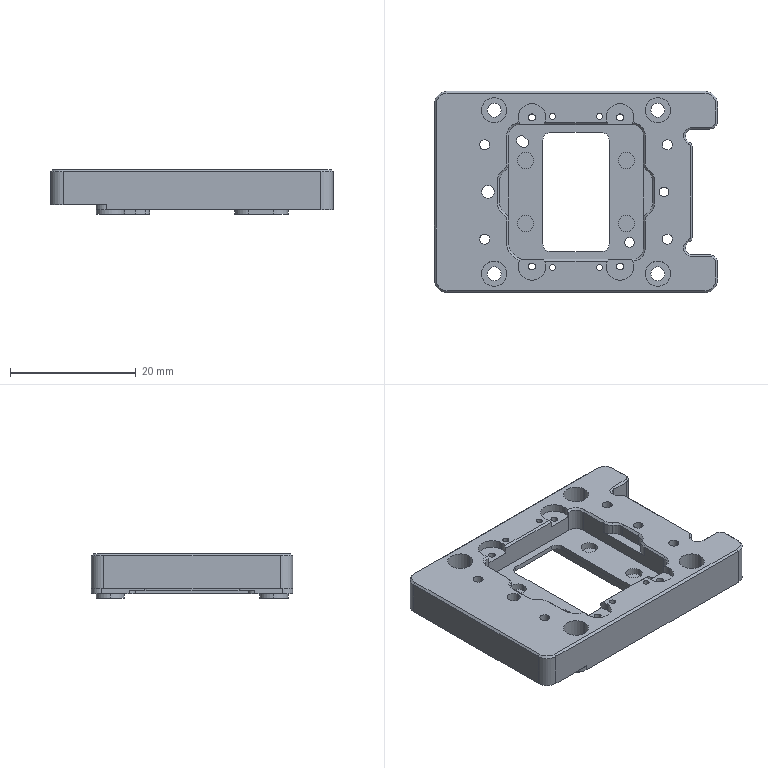NC program | NX | posted with a generic post | part box 45 x 32 x 7.05 mm
Lines 1 to 1919 of 2540, first 1706 of 1901 lines:
N10 G17 G21 G94 G90
(FLOOR_WALL_COPY , TOOL : D63)
N12 T03 M6
N14 G54
N16 G17 G0 G90 X-57. Y0. S6500 M3
N18 G43 Z30. H3
N20 Z5.
N22 G94 G1 Z2. F1250.
N24 X-54.
N26 X54.
N28 X57.
N30 Z5.
N32 G0 Z30.
N34 X-57.
N36 Z4.
N38 G1 Z1.
N40 X-54.
N42 X54.
N44 X57.
N46 Z4.
N48 G0 Z30.
N50 X-57.
N52 Z3.
N54 G1 Z0.
N56 X-54.
N58 X54.
N60 X57.
N62 Z3.
N64 G0 Z30.
N66 M5
(DRILLING_COPY_1 , TOOL : D6A45)
N68 T01 M6
N70 G54
N72 G17 G0 G90 X8.987 Y12.964 S5000 M3
N74 G43 Z30. H1
N76 G94 G81 G98 Z-0.6 F250. R3.
N78 X-9.013 Y-13.028
N80 G80
N82 G0 X-9.013 Y-13.028 Z30.
N84 M5
(DRILLING_COPY_COPY_1_COPY_COPY_1 , TOOL : 1.17ZT)
N86 T18 M6
N88 G54
N90 G17 G0 G90 X8.987 Y12.964 S2000 M3
N92 G43 Z30. H18
N94 G94 G83 G98 Z-3.352 F100. Q1. R3.
N96 X-9.013 Y-13.028
N98 G80
N100 G0 X-9.013 Y-13.028 Z30.
N102 M5
(FLOOR_WALL_2 , TOOL : D6)
N104 T06 M6
N106 G54
N108 G17 G0 G90 X1.501 Y-21.097 S9500 M3
N110 G43 Z30. H6
N112 Z0.7
N114 G94 G1 Z-0.3 F1000.
N116 X0.52 Y-19.397
N118 G3 X0. Y-19.097 R0.6
N120 G1 X-20.5 F2500.
N122 G2 X-25.597 Y-14. R5.097
N124 G1 Y-11.214
N126 G2 X-24.397 Y-8.317 R4.097
N128 G1 X-24.183 Y-8.103
N130 G2 X-21.597 Y-6.915 R4.097
N132 G1 Y6.915
N134 G2 X-24.183 Y8.103 R4.097
N136 G1 X-24.397 Y8.317
N138 G2 X-25.597 Y11.214 R4.097
N140 G1 Y14.
N142 G2 X-20.5 Y19.097 R5.097
N144 G1 X20.5
N146 G2 X25.597 Y14. R5.097
N148 G1 Y-14.
N150 G2 X20.5 Y-19.097 R5.097
N152 G1 X0.
N154 Y-16.097
N156 X-3.94
N158 G3 X-3.309 Y-11.355 R5.95
N160 X-3.948 Y-10.105 R3.7
N162 X-4.701 Y-8.92 R3.7
N164 X-9.025 Y-7.058 R5.95
N166 G1 X-13.025
N168 G3 X-18.11 Y-16.097 R5.95
N170 G1 X-17.597 Y-15.786
N172 G2 X-13.025 Y-7.658 R5.35
N174 G1 X-9.025
N176 G2 X-5.137 Y-9.332 R5.35
N178 X-4.475 Y-10.406 R3.1
N180 X-3.886 Y-11.521 R3.1
N182 X-9.025 Y-18.358 R5.35
N184 G1 X-13.025
N186 G2 X-17.597 Y-15.786 R5.35
N188 G1 X-18.11 Y-16.097
N190 X-20.5
N192 G2 X-22.597 Y-14. R2.097
N194 G1 Y-11.214
N196 G2 X-22.276 Y-10.439 R1.097
N198 G1 X-22.061 Y-10.224
N200 G2 X-21.369 Y-9.906 R1.097
N202 G3 X-18.597 Y-6.915 R3.
N204 G1 Y6.915
N206 G3 X-21.369 Y9.906 R3.
N208 G2 X-22.061 Y10.224 R1.097
N210 G1 X-22.276 Y10.439
N212 G2 X-22.597 Y11.214 R1.097
N214 G1 Y14.
N216 G2 X-20.5 Y16.097 R2.097
N218 G1 X-18.098
N220 G3 X-7.953 Y16.097 R-5.95
N222 G1 X-8.464 Y15.783
N224 G2 X-10.23 Y8.426 R5.35
N226 X-8.464 Y15.783 R-5.35
N228 G1 X-7.953 Y16.097
N230 X3.912
N232 G3 X3.257 Y11.359 R5.95
N234 X3.907 Y10.083 R3.7
N236 X4.677 Y8.874 R3.7
N238 X8.981 Y7.032 R5.95
N240 G1 X12.981
N242 G3 X18.051 Y16.097 R5.95
N244 G1 X17.54 Y15.783
N246 G2 X12.981 Y7.632 R5.35
N248 G1 X8.981
N250 G2 X5.111 Y9.288 R5.35
N252 X4.435 Y10.384 R3.1
N254 X3.834 Y11.523 R3.1
N256 X8.981 Y18.332 R5.35
N258 G1 X12.981
N260 G2 X17.54 Y15.783 R5.35
N262 G1 X18.051 Y16.097
N264 X20.5
N266 G2 X22.597 Y14. R2.097
N268 G1 Y-14.
N270 G2 X20.5 Y-16.097 R2.097
N272 G1 X18.063
N274 G3 X7.888 Y-16.097 R-5.95
N276 G1 X8.401 Y-15.786
N278 G2 X10.201 Y-8.437 R5.35
N280 X8.401 Y-15.786 R-5.35
N282 G1 X7.888 Y-16.097
N284 X0.
N286 Y-13.097
N288 X-0.075
N290 G3 X-0.427 Y-10.521 R8.95
N292 X-1.329 Y-8.607 R6.7
N294 X-2.522 Y-6.859 R6.7
N296 X-9.025 Y-4.058 R8.95
N298 G1 X-13.025
N300 G3 X-15.597 Y-4.436 R8.95
N302 G1 Y4.415
N304 G3 X-4.076 Y12.987 R8.95
N306 G1 Y13.097
N308 X0.032
N310 G3 X0.371 Y10.541 R8.95
N312 X1.287 Y8.585 R6.7
N314 X2.507 Y6.803 R6.7
N316 X8.981 Y4.032 R8.95
N318 G1 X12.981
N320 G3 X19.597 Y6.954 R8.95
N322 G1 Y-6.989
N324 G3 X4.026 Y-13.011 R8.95
N326 G1 Y-13.097
N328 X0.
N330 X1.965 Y-8.365
N332 G3 X1.281 Y-7.114 R9.7
N334 X-0.342 Y-4.798 R9.7
N336 X-9.025 Y-1.058 R11.95
N338 G1 X-12.597
N340 Y1.045
N342 G3 X-2.012 Y8.35 R11.95
N344 X-1.323 Y7.093 R9.7
N346 X0.337 Y4.731 R9.7
N348 X8.981 Y1.032 R11.95
N350 G1 X12.981
N352 G3 X16.597 Y1.592 R11.95
N354 G1 Y-1.623
N356 G3 X1.965 Y-8.365 R11.95
N358 G1 X1.976 Y-2.886
N360 G3 X-3.997 Y1.071 R14.95
N362 X-2.024 Y2.865 R14.95
N364 X-1.833 Y2.66 R12.7
N366 X3.947 Y-1.095 R14.95
N368 X1.976 Y-2.886 R14.95
N370 X1.845 Y-3.471 R0.6
N372 G1 Z0.7
N374 G0 X1.501 Y-21.097 Z0.4
N376 G1 Z-0.6 F1000.
N378 X0.52 Y-19.397
N380 G3 X0. Y-19.097 R0.6
N382 G1 X-20.5 F2500.
N384 G2 X-25.597 Y-14. R5.097
N386 G1 Y-11.214
N388 G2 X-24.397 Y-8.317 R4.097
N390 G1 X-24.183 Y-8.103
N392 G2 X-21.597 Y-6.915 R4.097
N394 G1 Y6.915
N396 G2 X-24.183 Y8.103 R4.097
N398 G1 X-24.397 Y8.317
N400 G2 X-25.597 Y11.214 R4.097
N402 G1 Y14.
N404 G2 X-20.5 Y19.097 R5.097
N406 G1 X20.5
N408 G2 X25.597 Y14. R5.097
N410 G1 Y-14.
N412 G2 X20.5 Y-19.097 R5.097
N414 G1 X0.
N416 Y-16.097
N418 X-3.94
N420 G3 X-3.309 Y-11.355 R5.95
N422 X-3.948 Y-10.105 R3.7
N424 X-4.701 Y-8.92 R3.7
N426 X-9.025 Y-7.058 R5.95
N428 G1 X-13.025
N430 G3 X-18.11 Y-16.097 R5.95
N432 G1 X-17.597 Y-15.786
N434 G2 X-13.025 Y-7.658 R5.35
N436 G1 X-9.025
N438 G2 X-5.137 Y-9.332 R5.35
N440 X-4.475 Y-10.406 R3.1
N442 X-3.886 Y-11.521 R3.1
N444 X-9.025 Y-18.358 R5.35
N446 G1 X-13.025
N448 G2 X-17.597 Y-15.786 R5.35
N450 G1 X-18.11 Y-16.097
N452 X-20.5
N454 G2 X-22.597 Y-14. R2.097
N456 G1 Y-11.214
N458 G2 X-22.276 Y-10.439 R1.097
N460 G1 X-22.061 Y-10.224
N462 G2 X-21.369 Y-9.906 R1.097
N464 G3 X-18.597 Y-6.915 R3.
N466 G1 Y6.915
N468 G3 X-21.369 Y9.906 R3.
N470 G2 X-22.061 Y10.224 R1.097
N472 G1 X-22.276 Y10.439
N474 G2 X-22.597 Y11.214 R1.097
N476 G1 Y14.
N478 G2 X-20.5 Y16.097 R2.097
N480 G1 X-18.098
N482 G3 X-7.953 Y16.097 R-5.95
N484 G1 X-8.464 Y15.783
N486 G2 X-10.23 Y8.426 R5.35
N488 X-8.464 Y15.783 R-5.35
N490 G1 X-7.953 Y16.097
N492 X3.912
N494 G3 X3.257 Y11.359 R5.95
N496 X3.907 Y10.083 R3.7
N498 X4.677 Y8.874 R3.7
N500 X8.981 Y7.032 R5.95
N502 G1 X12.981
N504 G3 X18.051 Y16.097 R5.95
N506 G1 X17.54 Y15.783
N508 G2 X12.981 Y7.632 R5.35
N510 G1 X8.981
N512 G2 X5.111 Y9.288 R5.35
N514 X4.435 Y10.384 R3.1
N516 X3.834 Y11.523 R3.1
N518 X8.981 Y18.332 R5.35
N520 G1 X12.981
N522 G2 X17.54 Y15.783 R5.35
N524 G1 X18.051 Y16.097
N526 X20.5
N528 G2 X22.597 Y14. R2.097
N530 G1 Y-14.
N532 G2 X20.5 Y-16.097 R2.097
N534 G1 X18.063
N536 G3 X7.888 Y-16.097 R-5.95
N538 G1 X8.401 Y-15.786
N540 G2 X10.201 Y-8.437 R5.35
N542 X8.401 Y-15.786 R-5.35
N544 G1 X7.888 Y-16.097
N546 X0.
N548 Y-13.097
N550 X-0.075
N552 G3 X-0.427 Y-10.521 R8.95
N554 X-1.329 Y-8.607 R6.7
N556 X-2.522 Y-6.859 R6.7
N558 X-9.025 Y-4.058 R8.95
N560 G1 X-13.025
N562 G3 X-15.597 Y-4.436 R8.95
N564 G1 Y4.415
N566 G3 X-4.076 Y12.987 R8.95
N568 G1 Y13.097
N570 X0.032
N572 G3 X0.371 Y10.541 R8.95
N574 X1.287 Y8.585 R6.7
N576 X2.507 Y6.803 R6.7
N578 X8.981 Y4.032 R8.95
N580 G1 X12.981
N582 G3 X19.597 Y6.954 R8.95
N584 G1 Y-6.989
N586 G3 X4.026 Y-13.011 R8.95
N588 G1 Y-13.097
N590 X0.
N592 X1.965 Y-8.365
N594 G3 X1.281 Y-7.114 R9.7
N596 X-0.342 Y-4.798 R9.7
N598 X-9.025 Y-1.058 R11.95
N600 G1 X-12.597
N602 Y1.045
N604 G3 X-2.012 Y8.35 R11.95
N606 X-1.323 Y7.093 R9.7
N608 X0.337 Y4.731 R9.7
N610 X8.981 Y1.032 R11.95
N612 G1 X12.981
N614 G3 X16.597 Y1.592 R11.95
N616 G1 Y-1.623
N618 G3 X1.965 Y-8.365 R11.95
N620 G1 X1.976 Y-2.886
N622 G3 X-3.997 Y1.071 R14.95
N624 X-2.024 Y2.865 R14.95
N626 X-1.833 Y2.66 R12.7
N628 X3.947 Y-1.095 R14.95
N630 X1.976 Y-2.886 R14.95
N632 X1.845 Y-3.471 R0.6
N634 G1 Z0.4
N636 G0 X27.597 Y1.501 Z0.15
N638 G1 Z-0.85 F1000.
N640 X25.897 Y0.52
N642 G3 X25.597 Y0. R0.6
N644 G1 Y-14. F2500.
N646 G2 X20.5 Y-19.097 R5.097
N648 G1 X14.187
N650 Y-19.067
N652 G3 X18.331 Y-14.4 R4.7
N654 G1 Y-10.
N656 G3 X14.231 Y-5.9 R4.1
N658 G1 X6.95
N660 G3 X2.85 Y-10. R4.1
N662 G1 Y-11.112
N664 G3 X0.281 Y-12.284 R4.1
N666 G2 X-0.281 Y-12.284 R0.4
N668 G3 X-2.85 Y-11.112 R4.1
N670 G1 Y11.112
N672 G3 X-0.281 Y12.284 R4.1
N674 G2 X0.281 Y12.284 R0.4
N676 G3 X2.85 Y11.112 R4.1
N678 G1 Y10.
N680 G3 X6.95 Y5.9 R4.1
N682 G1 X14.231
N684 G3 X18.331 Y10. R4.1
N686 G1 Y14.4
N688 G3 X14.187 Y19.067 R4.7
N690 G1 Y19.097
N692 X20.5
N694 G2 X25.597 Y14. R5.097
N696 G1 Y0.
N698 X22.597
N700 Y-14.
N702 G2 X21.166 Y-15.989 R2.097
N704 G3 X21.331 Y-14.4 R7.7
N706 G1 Y-10.
N708 G3 X14.231 Y-2.9 R7.1
N710 G1 X6.95
N712 G3 X0.15 Y-7.958 R7.1
N714 G1 Y7.958
N716 G3 X5.953 Y2.97 R7.1
N718 G1 X5.532 Y0.
N720 G3 X3.15 Y-0.642 R10.1
N722 G1 Y0.642
N724 G3 X5.532 Y0. R10.1
N726 G1 X5.953 Y2.97
N728 G3 X6.95 Y2.9 R7.1
N730 G1 X14.231
N732 G3 X21.331 Y10. R7.1
N734 G1 Y14.4
N736 G3 X21.166 Y15.989 R7.7
N738 G2 X22.597 Y14. R2.097
N740 G1 Y0.
N742 X19.597
N744 Y-1.443
N746 G3 X15.649 Y0. R10.1
N748 X19.597 Y1.443 R10.1
N750 G1 Y0.
N752 G3 X19.897 Y-0.52 R0.6
N754 G1 Z0.15
N756 G0 X27.597 Y1.501 Z-0.1
N758 G1 Z-1.1 F1000.
N760 X25.897 Y0.52
N762 G3 X25.597 Y0. R0.6
N764 G1 Y-14. F2500.
N766 G2 X20.5 Y-19.097 R5.097
N768 G1 X14.187
N770 Y-19.067
N772 G3 X18.331 Y-14.4 R4.7
N774 G1 Y-10.
N776 G3 X14.231 Y-5.9 R4.1
N778 G1 X6.95
N780 G3 X2.887 Y-9.453 R4.1
N782 X-2.85 Y-9.412 R3.85
N784 G1 Y9.412
N786 G3 X2.887 Y9.453 R3.85
N788 X6.95 Y5.9 R4.1
N790 G1 X14.231
N792 G3 X18.331 Y10. R4.1
N794 G1 Y14.4
N796 G3 X14.187 Y19.067 R4.7
N798 G1 Y19.097
N800 X20.5
N802 G2 X25.597 Y14. R5.097
N804 G1 Y0.
N806 X22.597
N808 Y-14.
N810 G2 X21.166 Y-15.989 R2.097
N812 G3 X21.331 Y-14.4 R7.7
N814 G1 Y-10.
N816 G3 X14.231 Y-2.9 R7.1
N818 G1 X6.95
N820 G3 X1.595 Y-5.338 R7.1
N822 X0.15 Y-5.152 R6.85
N824 G1 Y5.152
N826 G3 X1.595 Y5.338 R6.85
N828 X5.953 Y2.97 R7.1
N830 G1 X5.532 Y0.
N832 G3 X3.15 Y-0.642 R10.1
N834 G1 Y0.642
N836 G3 X5.532 Y0. R10.1
N838 G1 X5.953 Y2.97
N840 G3 X6.95 Y2.9 R7.1
N842 G1 X14.231
N844 G3 X21.331 Y10. R7.1
N846 G1 Y14.4
N848 G3 X21.166 Y15.989 R7.7
N850 G2 X22.597 Y14. R2.097
N852 G1 Y0.
N854 X19.597
N856 Y-1.443
N858 G3 X15.649 Y0. R10.1
N860 X19.597 Y1.443 R10.1
N862 G1 Y0.
N864 G3 X19.897 Y-0.52 R0.6
N866 G1 Z-0.1
N868 G0 X27.597 Y1.501 Z-0.4
N870 G1 Z-1.4 F1000.
N872 X25.897 Y0.52
N874 G3 X25.597 Y0. R0.6
N876 G1 Y-14. F2500.
N878 G2 X20.5 Y-19.097 R5.097
N880 G1 X14.187
N882 Y-19.067
N884 G3 X18.331 Y-14.4 R4.7
N886 G1 Y-7.824
N888 G3 X18.314 Y-7.5 R3.1
N890 X18.331 Y-7.176 R3.1
N892 G1 Y7.176
N894 G3 X18.314 Y7.5 R3.1
N896 X18.331 Y7.824 R3.1
N898 G1 Y14.4
N900 G3 X14.187 Y19.067 R4.7
N902 G1 Y19.097
N904 X20.5
N906 G2 X25.597 Y14. R5.097
N908 G1 Y0.
N910 X22.597
N912 Y-14.
N914 G2 X21.166 Y-15.989 R2.097
N916 G3 X21.331 Y-14.4 R7.7
N918 G1 Y-7.824
N920 G3 X21.323 Y-7.5 R6.1
N922 X21.331 Y-7.176 R6.1
N924 G1 Y7.176
N926 G3 X21.323 Y7.5 R6.1
N928 X21.331 Y7.824 R6.1
N930 G1 Y14.4
N932 G3 X21.166 Y15.989 R7.7
N934 G2 X22.597 Y14. R2.097
N936 G1 Y0.
N938 G3 X22.897 Y-0.52 R0.6
N940 G1 X27.597
N942 Z-0.4
N944 G0 Z30.
N946 X2.55
N948 Z-0.4
N950 G1 Z-1.4 F1000.
N952 G3 X2.85 Y0. R0.6
N954 G1 Y-9.412 F2500.
N956 G3 X-2.85 Y-9.412 R3.85
N958 G1 Y9.412
N960 G3 X2.85 Y9.412 R3.85
N962 G1 Y0.
N964 X0.15
N966 Y-5.452
N968 G3 X-0.15 Y-5.452 R6.55
N970 G1 Y5.452
N972 G3 X0.15 Y5.452 R6.55
N974 G1 Y0.
N976 G3 X0.45 Y-0.52 R0.6
N978 G1 Z-0.4
N980 G0 Z30.
N982 X-23.597 Y-1.501
N984 Z0.15
N986 G1 Z-0.85 F1000.
N988 X-21.897 Y-0.52
N990 G3 X-21.597 Y0. R0.6
N992 G1 Y6.912 F2500.
N994 G3 X-21.286 Y6.9 R4.1
N996 G1 X-19.394
N998 G3 X-16.711 Y5.9 R4.1
N1000 G1 X-12.464
N1002 Y-5.9
N1004 X-16.711
N1006 G3 X-19.394 Y-6.9 R4.1
N1008 G1 X-21.286
N1010 G3 X-21.597 Y-6.912 R4.1
N1012 G1 Y0.
N1014 X-18.597
N1016 Y3.155
N1018 G3 X-16.711 Y2.9 R7.1
N1020 G1 X-15.464
N1022 Y-2.9
N1024 X-16.711
N1026 G3 X-18.597 Y-3.155 R7.1
N1028 G1 Y0.
N1030 G3 X-18.897 Y0.52 R0.6
N1032 G1 X-23.597
N1034 Z0.15
N1036 G0 Y-1.501 Z-0.1
N1038 G1 Z-1.1 F1000.
N1040 X-21.897 Y-0.52
N1042 G3 X-21.597 Y0. R0.6
N1044 G1 Y6.912 F2500.
N1046 G3 X-21.286 Y6.9 R4.1
N1048 G1 X-19.394
N1050 G3 X-16.711 Y5.9 R4.1
N1052 G1 X-12.464
N1054 Y-5.9
N1056 X-16.711
N1058 G3 X-19.394 Y-6.9 R4.1
N1060 G1 X-21.286
N1062 G3 X-21.597 Y-6.912 R4.1
N1064 G1 Y0.
N1066 X-18.597
N1068 Y3.155
N1070 G3 X-16.711 Y2.9 R7.1
N1072 G1 X-15.464
N1074 Y-2.9
N1076 X-16.711
N1078 G3 X-18.597 Y-3.155 R7.1
N1080 G1 Y0.
N1082 G3 X-18.897 Y0.52 R0.6
N1084 G1 X-23.597
N1086 Z-0.1
N1088 G0 Z30.
N1090 X-2.55
N1092 Z-1.05
N1094 G1 Z-2.05 F1000.
N1096 G3 X-2.85 Y0. R0.6
N1098 G1 Y9.412 F2500.
N1100 G3 X2.85 Y9.412 R3.85
N1102 G1 Y-9.412
N1104 G3 X-2.85 Y-9.412 R3.85
N1106 G1 Y0.
N1108 X-0.15
N1110 Y5.452
N1112 G3 X0.15 Y5.452 R6.55
N1114 G1 Y-5.452
N1116 G3 X-0.15 Y-5.452 R6.55
N1118 G1 Y0.
N1120 G3 X-0.45 Y0.52 R0.6
N1122 G1 Z-1.05
N1124 G0 X-2.55 Z-1.35
N1126 G1 Z-2.35 F1000.
N1128 G3 X-2.85 Y0. R0.6
N1130 G1 Y9.412 F2500.
N1132 G3 X2.85 Y9.412 R3.85
N1134 G1 Y-9.412
N1136 G3 X-2.85 Y-9.412 R3.85
N1138 G1 Y0.
N1140 X-0.15
N1142 Y5.452
N1144 G3 X0.15 Y5.452 R6.55
N1146 G1 Y-5.452
N1148 G3 X-0.15 Y-5.452 R6.55
N1150 G1 Y0.
N1152 G3 X-0.45 Y0.52 R0.6
N1154 G1 Z-1.35
N1156 G0 Z30.
N1158 M5
(CAVITY_MILL_COPY_1 , TOOL : D3)
N1160 T17 M6
N1162 G54
N1164 G17 G0 G90 X-13.36 Y-6.9 S9500 M3
N1166 G43 Z30. H17
N1168 Z-0.95
N1170 G94 G1 X-13.302 Y-7. F1100.
N1172 G3 X-12.436 Y-7.5 R1.
N1174 G1 X-10.864
N1176 Y-5.928
N1178 G3 X-11.364 Y-5.062 R1.
N1180 G1 X-11.464 Y-5.005
N1182 G0 X-13.36 Y-6.9 Z-1.2
N1184 G1 X-13.302 Y-7.
N1186 G3 X-12.436 Y-7.5 R1.
N1188 G1 X-10.864
N1190 Y-5.928
N1192 G3 X-11.364 Y-5.062 R1.
N1194 G1 X-11.464 Y-5.005
N1196 G0 Z30.
N1198 Y5.005
N1200 Z-0.95
N1202 G1 X-11.364 Y5.062
N1204 G3 X-10.864 Y5.928 R1.
N1206 G1 Y7.5
N1208 X-12.436
N1210 G3 X-13.302 Y7. R1.
N1212 G1 X-13.36 Y6.9
N1214 G0 X-11.464 Y5.005 Z-1.2
N1216 G1 X-11.364 Y5.062
N1218 G3 X-10.864 Y5.928 R1.
N1220 G1 Y7.5
N1222 X-12.436
N1224 G3 X-13.302 Y7. R1.
N1226 G1 X-13.36 Y6.9
N1228 G0 Z30.
(CAVITY_MILL_COPY_1_COPY , TOOL : D3)
N1230 X-1.435 Y9.605
N1232 Z-0.992
N1234 G3 X-1.644 Y10.55 R1.
N1236 G2 X-1.94 Y13.02 R2.192
N1238 X-3.164 Y12.7 R2.5
N1240 G1 X-4.25
N1242 G3 X-4.45 Y12.5 R0.2
N1244 G1 Y9.709
N1246 G3 X-3.95 Y8.843 R1.
N1248 G1 X-3.85 Y8.785
N1250 G0 X-1.436 Y9.538 Z-1.283
N1252 G3 X-1.661 Y10.482 R1.
N1254 G2 X-2.029 Y12.972 R2.25
N1256 X-3.164 Y12.7 R2.5
N1258 G1 X-4.25
N1260 G3 X-4.45 Y12.5 R0.2
N1262 G1 Y9.613
N1264 G3 X-3.95 Y8.747 R1.
N1266 G1 X-3.85 Y8.69
N1268 G0 X-1.436 Y9.538 Z-1.575
N1270 G3 X-1.661 Y10.482 R1.
N1272 G2 X-2.029 Y12.972 R2.25
N1274 X-3.164 Y12.7 R2.5
N1276 G1 X-4.25
N1278 G3 X-4.45 Y12.5 R0.2
N1280 G1 Y9.613
N1282 G3 X-3.95 Y8.747 R1.
N1284 G1 X-3.85 Y8.69
N1286 G0 X-1.436 Y9.538 Z-1.867
N1288 G3 X-1.661 Y10.482 R1.
N1290 G2 X-2.029 Y12.972 R2.25
N1292 X-3.164 Y12.7 R2.5
N1294 G1 X-4.25
N1296 G3 X-4.45 Y12.5 R0.2
N1298 G1 Y9.613
N1300 G3 X-3.95 Y8.747 R1.
N1302 G1 X-3.85 Y8.69
N1304 G0 X-1.436 Y9.538 Z-2.158
N1306 G3 X-1.661 Y10.482 R1.
N1308 G2 X-2.029 Y12.972 R2.25
N1310 X-3.164 Y12.7 R2.5
N1312 G1 X-4.25
N1314 G3 X-4.45 Y12.5 R0.2
N1316 G1 Y9.613
N1318 G3 X-3.95 Y8.747 R1.
N1320 G1 X-3.85 Y8.69
N1322 G0 X-1.436 Y9.538 Z-2.45
N1324 G3 X-1.661 Y10.482 R1.
N1326 G2 X-2.029 Y12.972 R2.25
N1328 X-3.164 Y12.7 R2.5
N1330 G1 X-4.25
N1332 G3 X-4.45 Y12.5 R0.2
N1334 G1 Y9.613
N1336 G3 X-3.95 Y8.747 R1.
N1338 G1 X-3.85 Y8.69
N1340 G0 Z30.
N1342 X4.077 Y8.836
N1344 Z-0.992
N1346 G3 X4.464 Y9.736 R1.
N1348 G2 X4.45 Y10. R2.5
N1350 G1 Y12.5
N1352 G3 X4.25 Y12.7 R0.2
N1354 G1 X3.164
N1356 G2 X1.94 Y13.02 R2.5
N1358 X1.647 Y10.554 R2.192
N1360 G3 X1.441 Y9.609 R1.
N1362 G0 X3.85 Y8.69 Z-1.283
N1364 G1 X3.95 Y8.747
N1366 G3 X4.45 Y9.613 R1.
N1368 G1 Y12.5
N1370 G3 X4.25 Y12.7 R0.2
N1372 G1 X3.164
N1374 G2 X2.029 Y12.972 R2.5
N1376 X1.661 Y10.482 R2.25
N1378 G3 X1.436 Y9.538 R1.
N1380 G0 X3.85 Y8.69 Z-1.575
N1382 G1 X3.95 Y8.747
N1384 G3 X4.45 Y9.613 R1.
N1386 G1 Y12.5
N1388 G3 X4.25 Y12.7 R0.2
N1390 G1 X3.164
N1392 G2 X2.029 Y12.972 R2.5
N1394 X1.661 Y10.482 R2.25
N1396 G3 X1.436 Y9.538 R1.
N1398 G0 X3.85 Y8.69 Z-1.867
N1400 G1 X3.95 Y8.747
N1402 G3 X4.45 Y9.613 R1.
N1404 G1 Y12.5
N1406 G3 X4.25 Y12.7 R0.2
N1408 G1 X3.164
N1410 G2 X2.029 Y12.972 R2.5
N1412 X1.661 Y10.482 R2.25
N1414 G3 X1.436 Y9.538 R1.
N1416 G0 X3.85 Y8.69 Z-2.158
N1418 G1 X3.95 Y8.747
N1420 G3 X4.45 Y9.613 R1.
N1422 G1 Y12.5
N1424 G3 X4.25 Y12.7 R0.2
N1426 G1 X3.164
N1428 G2 X2.029 Y12.972 R2.5
N1430 X1.661 Y10.482 R2.25
N1432 G3 X1.436 Y9.538 R1.
N1434 G0 X3.85 Y8.69 Z-2.45
N1436 G1 X3.95 Y8.747
N1438 G3 X4.45 Y9.613 R1.
N1440 G1 Y12.5
N1442 G3 X4.25 Y12.7 R0.2
N1444 G1 X3.164
N1446 G2 X2.029 Y12.972 R2.5
N1448 X1.661 Y10.482 R2.25
N1450 G3 X1.436 Y9.538 R1.
N1452 G0 Z30.
N1454 X1.441 Y-9.609
N1456 Z-0.992
N1458 G3 X1.647 Y-10.554 R1.
N1460 G2 X1.94 Y-13.02 R2.192
N1462 X3.164 Y-12.7 R2.5
N1464 G1 X3.629
N1466 X3.717 Y-12.712
N1468 X3.77 Y-12.641
N1470 X4.391 Y-12.02
N1472 X4.462 Y-11.967
N1474 X4.45 Y-11.879
N1476 Y-10.
N1478 G2 X4.464 Y-9.736 R2.5
N1480 G3 X4.077 Y-8.836 R1.
N1482 G0 X1.436 Y-9.538 Z-1.283
N1484 G3 X1.661 Y-10.482 R1.
N1486 G2 X2.056 Y-12.915 R2.25
N1488 G1 X2.04 Y-12.967
N1490 G2 X3.164 Y-12.7 R2.5
N1492 G1 X3.629
N1494 X3.717 Y-12.712
N1496 X3.77 Y-12.641
N1498 X4.391 Y-12.02
N1500 X4.462 Y-11.967
N1502 X4.45 Y-11.879
N1504 Y-9.613
N1506 G3 X3.95 Y-8.747 R1.
N1508 G1 X3.85 Y-8.69
N1510 G0 X1.436 Y-9.538 Z-1.575
N1512 G3 X1.661 Y-10.482 R1.
N1514 G2 X2.056 Y-12.915 R2.25
N1516 G1 X2.041 Y-12.966
N1518 G2 X3.164 Y-12.7 R2.5
N1520 G1 X3.629
N1522 X3.717 Y-12.712
N1524 X3.77 Y-12.641
N1526 X4.391 Y-12.02
N1528 X4.462 Y-11.967
N1530 X4.45 Y-11.879
N1532 Y-9.613
N1534 G3 X3.95 Y-8.747 R1.
N1536 G1 X3.85 Y-8.69
N1538 G0 X1.436 Y-9.538 Z-1.867
N1540 G3 X1.661 Y-10.482 R1.
N1542 G2 X2.056 Y-12.915 R2.25
N1544 G1 X2.042 Y-12.966
N1546 G2 X3.164 Y-12.7 R2.5
N1548 G1 X3.629
N1550 X3.717 Y-12.712
N1552 X3.77 Y-12.641
N1554 X4.391 Y-12.02
N1556 X4.462 Y-11.967
N1558 X4.45 Y-11.879
N1560 Y-9.613
N1562 G3 X3.95 Y-8.747 R1.
N1564 G1 X3.85 Y-8.69
N1566 G0 X1.436 Y-9.538 Z-2.158
N1568 G3 X1.661 Y-10.482 R1.
N1570 G2 X2.038 Y-12.954 R2.25
N1572 G1 X2.043 Y-12.965
N1574 G2 X3.164 Y-12.7 R2.5
N1576 G1 X3.629
N1578 X3.717 Y-12.712
N1580 X3.77 Y-12.641
N1582 X4.391 Y-12.02
N1584 X4.462 Y-11.967
N1586 X4.45 Y-11.879
N1588 Y-9.613
N1590 G3 X3.95 Y-8.747 R1.
N1592 G1 X3.85 Y-8.69
N1594 G0 X1.436 Y-9.538 Z-2.45
N1596 G3 X1.661 Y-10.482 R1.
N1598 G2 X2.038 Y-12.954 R2.25
N1600 G1 X2.044 Y-12.965
N1602 G2 X3.164 Y-12.7 R2.5
N1604 G1 X3.629
N1606 X3.717 Y-12.712
N1608 X3.77 Y-12.641
N1610 X4.391 Y-12.02
N1612 X4.462 Y-11.967
N1614 X4.45 Y-11.879
N1616 Y-9.613
N1618 G3 X3.95 Y-8.747 R1.
N1620 G1 X3.85 Y-8.69
N1622 G0 Z30.
N1624 X-3.85 Y-8.785
N1626 Z-0.992
N1628 G1 X-3.95 Y-8.843
N1630 G3 X-4.45 Y-9.709 R1.
N1632 G1 Y-12.5
N1634 G3 X-4.25 Y-12.7 R0.2
N1636 G1 X-3.164
N1638 G2 X-1.94 Y-13.02 R2.5
N1640 X-1.644 Y-10.55 R2.192
N1642 G3 X-1.435 Y-9.605 R1.
N1644 G0 X-3.85 Y-8.69 Z-1.283
N1646 G1 X-3.95 Y-8.747
N1648 G3 X-4.45 Y-9.613 R1.
N1650 G1 Y-12.5
N1652 G3 X-4.25 Y-12.7 R0.2
N1654 G1 X-3.164
N1656 G2 X-2.04 Y-12.967 R2.5
N1658 G1 X-2.056 Y-12.915
N1660 G2 X-1.661 Y-10.482 R2.25
N1662 G3 X-1.436 Y-9.538 R1.
N1664 G0 X-3.85 Y-8.69 Z-1.575
N1666 G1 X-3.95 Y-8.747
N1668 G3 X-4.45 Y-9.613 R1.
N1670 G1 Y-12.5
N1672 G3 X-4.25 Y-12.7 R0.2
N1674 G1 X-3.164
N1676 G2 X-2.041 Y-12.966 R2.5
N1678 G1 X-2.056 Y-12.915
N1680 G2 X-1.661 Y-10.482 R2.25
N1682 G3 X-1.436 Y-9.538 R1.
N1684 G0 X-3.85 Y-8.69 Z-1.867
N1686 G1 X-3.95 Y-8.747
N1688 G3 X-4.45 Y-9.613 R1.
N1690 G1 Y-12.5
N1692 G3 X-4.25 Y-12.7 R0.2
N1694 G1 X-3.164
N1696 G2 X-2.042 Y-12.966 R2.5
N1698 G1 X-2.056 Y-12.915
N1700 G2 X-1.661 Y-10.482 R2.25
N1702 G3 X-1.436 Y-9.538 R1.
N1704 G0 X-3.85 Y-8.69 Z-2.158
N1706 G1 X-3.95 Y-8.747
N1708 G3 X-4.45 Y-9.613 R1.
N1710 G1 Y-12.5
N1712 G3 X-4.25 Y-12.7 R0.2
N1714 G1 X-3.164
N1716 G2 X-2.043 Y-12.965 R2.5
N1718 G1 X-2.038 Y-12.954
N1720 G2 X-1.661 Y-10.482 R2.25
N1722 G3 X-1.436 Y-9.538 R1.
N1724 G0 X-3.85 Y-8.69 Z-2.45
N1726 G1 X-3.95 Y-8.747
N1728 G3 X-4.45 Y-9.613 R1.
N1730 G1 Y-12.5
N1732 G3 X-4.25 Y-12.7 R0.2
N1734 G1 X-3.164
N1736 G2 X-2.044 Y-12.965 R2.5
N1738 G1 X-2.038 Y-12.954
N1740 G2 X-1.661 Y-10.482 R2.25
N1742 G3 X-1.436 Y-9.538 R1.
N1744 G0 Z30.
(FLOOR_WALL_1_COPY_COPY , TOOL : D3)
N1746 X25. Y0.751
N1748 Z-0.5
N1750 G1 Z-1.5 F1000.
N1752 X24.15 Y0.26
N1754 G3 X24. Y0. R0.3
N1756 G1 Y-14.
N1758 G2 X20.5 Y-17.5 R3.5
N1760 G1 X14.607
N1762 G3 X16.881 Y-14.4 R3.25
N1764 G1 Y-7.824
N1766 G3 X16.849 Y-7.5 R1.65
N1768 X16.881 Y-7.176 R1.65
N1770 G1 Y7.176
N1772 G3 X16.849 Y7.5 R1.65
N1774 X16.881 Y7.824 R1.65
N1776 G1 Y14.4
N1778 G3 X14.607 Y17.5 R3.25
N1780 G1 X20.5
N1782 G2 X24. Y14. R3.5
N1784 G1 Y0.
N1786 X22.5
N1788 Y-14.
N1790 G2 X20.5 Y-16. R2.
N1792 G1 X18.104
N1794 G3 X18.381 Y-14.4 R4.75
N1796 G1 Y-7.824
N1798 G3 X18.365 Y-7.5 R3.15
N1800 X18.381 Y-7.176 R3.15
N1802 G1 Y7.176
N1804 G3 X18.365 Y7.5 R3.15
N1806 X18.381 Y7.824 R3.15
N1808 G1 Y14.4
N1810 G3 X18.104 Y16. R4.75
N1812 G1 X20.5
N1814 G2 X22.5 Y14. R2.
N1816 G1 Y0.
N1818 X21.
N1820 Y-14.
N1822 G2 X20.5 Y-14.5 R0.5
N1824 G1 X19.88
N1826 X19.881 Y-14.4
N1828 Y-7.824
N1830 G3 X19.87 Y-7.5 R4.65
N1832 X19.881 Y-7.176 R4.65
N1834 G1 Y7.176
N1836 G3 X19.87 Y7.5 R4.65
N1838 X19.881 Y7.824 R4.65
N1840 G1 Y14.4
N1842 X19.88 Y14.5
N1844 X20.5
N1846 G2 X21. Y14. R0.5
N1848 G1 Y0.
N1850 G3 X21.15 Y-0.26 R0.3
N1852 G1 Z-0.5
N1854 G0 Z30.
N1856 X13.235 Y18.5
N1858 Z-0.5
N1860 G1 Z-1.5
N1862 X13.633 Y17.66
N1864 G3 X13.88 Y17.49 R0.3
N1866 G2 X16.731 Y14.4 R3.1
N1868 G1 Y7.824
N1870 G2 X16.696 Y7.5 R1.5
N1872 X16.731 Y7.176 R1.5
N1874 G1 Y-7.176
N1876 G2 X16.696 Y-7.5 R1.5
N1878 X16.731 Y-7.824 R1.5
N1880 G1 Y-14.4
N1882 G2 X13.88 Y-17.49 R3.1
N1884 G3 X13.633 Y-17.66 R0.3
N1886 G1 X13.235 Y-18.5
N1888 Z-0.5
N1890 G0 Z30.
N1892 X17.731 Y0.751
N1894 Z-0.2
N1896 G1 Z-1.2
N1898 X16.881 Y0.26
N1900 G3 X16.731 Y0. R0.3
N1902 G1 Y-9.121
N1904 G3 X14.231 Y-7.35 R2.65
N1906 G1 X6.95
N1908 G3 X4.45 Y-9.121 R2.65
N1910 G1 Y9.121
N1912 G3 X6.95 Y7.35 R2.65
N1914 G1 X14.231
N1916 G3 X16.731 Y9.121 R2.65
N1918 G1 Y0.
N1920 X15.231
N1922 Y-5.972
N1924 G3 X14.231 Y-5.85 R4.15
N1926 G1 X6.95
N1928 G3 X5.95 Y-5.972 R4.15
N1930 G1 Y5.972
N1932 G3 X6.95 Y5.85 R4.15
N1934 G1 X14.231
N1936 G3 X15.231 Y5.972 R4.15
N1938 G1 Y0.
N1940 X13.731
N1942 Y-4.35
N1944 X7.45
N1946 Y4.35
N1948 X13.731
N1950 Y0.
N1952 X12.231
N1954 Y-2.85
N1956 X8.95
N1958 Y2.85
N1960 X12.231
N1962 Y0.
N1964 X10.731
N1966 Y-1.35
N1968 X10.45
N1970 Y1.35
N1972 X10.731
N1974 Y0.
N1976 G3 X10.881 Y-0.26 R0.3
N1978 G1 Z-0.2
N1980 G0 Z30.
N1982 X17.731 Y10.41
N1984 Z-0.2
N1986 G1 Z-1.2
N1988 X16.894 Y10.022
N1990 G3 X16.721 Y9.777 R0.3
N1992 G2 X14.231 Y7.5 R2.5
N1994 G1 X6.95
N1996 G2 X4.46 Y9.777 R2.5
N1998 G3 X4.287 Y10.022 R0.3
N2000 G1 X3.45 Y10.41
N2002 Z-0.2
N2004 G0 Z30.
N2006 Y-10.41
N2008 Z-0.2
N2010 G1 Z-1.2
N2012 X4.287 Y-10.022
N2014 G3 X4.46 Y-9.777 R0.3
N2016 G2 X6.95 Y-7.5 R2.5
N2018 G1 X14.231
N2020 G2 X16.721 Y-9.777 R2.5
N2022 G3 X16.894 Y-10.022 R0.3
N2024 G1 X17.731 Y-10.41
N2026 Z-0.2
N2028 G0 Z30.
N2030 X-0.704 Y-8.93
N2032 Z0.05
N2034 G1 Z-0.95
N2036 X-0.26 Y-9.7
N2038 G3 X0. Y-9.85 R0.3
N2040 G2 X1.939 Y-12.928 R2.15
N2042 G1 X1.892 Y-12.902
N2044 X1.838 Y-12.904
N2046 X1.792 Y-12.932
N2048 G3 X1.301 Y-13.316 R2.65
N2050 G2 X-1.301 Y-13.316 R1.85
N2052 G3 X-1.792 Y-12.932 R2.65
N2054 G1 X-1.838 Y-12.904
N2056 X-1.892 Y-12.902
N2058 X-1.939 Y-12.928
N2060 G2 X0. Y-9.85 R2.15
N2062 G1 Y-11.35
N2064 G2 X0.643 Y-11.904 R0.65
N2066 G3 X0.246 Y-12.249 R4.15
N2068 G2 X-0.246 Y-12.249 R0.35
N2070 G3 X-0.643 Y-11.904 R4.15
N2072 G2 X0. Y-11.35 R0.65
N2074 G3 X0.26 Y-11.2 R0.3
N2076 G1 X0.973 Y-9.004
N2078 Z0.05
N2080 G0 Z30.
N2082 X-1.138 Y-12.164
N2084 Z0.05
N2086 G1 Z-0.95
N2088 X-2.015 Y-12.798
N2090 G3 X-1.87 Y-13.061 R0.3
N2092 G2 X-1.406 Y-13.422 R2.5
N2094 G3 X1.406 Y-13.422 R2.
N2096 G2 X1.87 Y-13.061 R2.5
N2098 G3 X2.015 Y-12.798 R0.3
N2100 G1 X1.138 Y-12.164
N2102 Z0.05
N2104 G0 Z30.
N2106 X-21. Y-0.751
N2108 Z-0.2
N2110 G1 Z-1.2
N2112 X-20.15 Y-0.26
N2114 G3 X-20. Y0. R0.3
N2116 G1 Y7.053
N2118 G2 X-19.622 Y8.375 R2.5
N2120 G1 X-19.585 Y8.347
N2122 X-19.539 Y8.35
N2124 X-18.785
N2126 G3 X-16.711 Y7.35 R2.65
N2128 G1 X-11.014
N2130 Y-7.35
N2132 X-16.711
N2134 G3 X-18.785 Y-8.35 R2.65
N2136 G1 X-19.539
N2138 X-19.585 Y-8.347
N2140 X-19.622 Y-8.375
N2142 G2 X-20. Y-7.053 R2.5
N2144 G1 Y0.
N2146 X-18.5
N2148 Y6.255
N2150 G3 X-16.711 Y5.85 R4.15
N2152 G1 X-12.514
N2154 Y-5.85
N2156 X-16.711
N2158 G3 X-18.5 Y-6.255 R4.15
N2160 G1 Y0.
N2162 X-17.
N2164 Y4.357
N2166 G3 X-16.711 Y4.35 R5.65
N2168 G1 X-14.014
N2170 Y-4.35
N2172 X-16.711
N2174 G3 X-17. Y-4.357 R5.65
N2176 G1 Y0.
N2178 X-15.65
N2180 Y3.
N2182 X-15.364
N2184 Y-3.
N2186 X-15.65
N2188 Y0.
N2190 G3 X-15.8 Y0.26 R0.3
N2192 G1 Z-0.2
N2194 G0 Z30.
N2196 X-18.997 Y-7.154
N2198 Z-0.2
N2200 G1 Z-1.2
N2202 X-19.799 Y-8.35
N2204 G3 X-19.539 Y-8.5 R0.3
N2206 G1 X-18.711
N2208 G2 X-16.711 Y-7.5 R2.5
N2210 G1 X-10.864
N2212 Y7.5
N2214 X-16.711
N2216 G2 X-18.711 Y8.5 R2.5
N2218 G1 X-19.539
N2220 G3 X-19.799 Y8.35 R0.3
N2222 G1 X-18.997 Y7.154
N2224 Z-0.2
N2226 G0 Z30.
N2228 X-3.45 Y2.887
N2230 Z0.3
N2232 G1 Z-0.7
N2234 X-4.3 Y2.396
N2236 G3 X-4.45 Y2.137 R0.3
N2238 G1 Y-12.5
N2240 G3 X-4.25 Y-12.7 R0.2
N2242 G1 X-3.164
N2244 G2 X-1.406 Y-13.422 R2.5
N2246 G3 X1.406 Y-13.422 R2.
N2248 G2 X3.164 Y-12.7 R2.5
N2250 G1 X3.629
N2252 X3.683 Y-12.703
N2254 X3.734 Y-12.682
N2256 X3.77 Y-12.641
N2258 X4.391 Y-12.02
N2260 X4.432 Y-11.984
N2262 X4.453 Y-11.933
N2264 X4.45 Y-11.879
N2266 Y-10.
N2268 G2 X6.95 Y-7.5 R2.5
N2270 G1 X14.231
N2272 G2 X16.731 Y-10. R2.5
N2274 G1 Y-11.96
N2276 G3 X16.731 Y-14.062 R-3.9
N2278 G1 Y-14.4
N2280 G2 X13.631 Y-17.5 R3.1
N2282 G1 X-6.077
N2284 Y-16.
N2286 G3 X-4.955 Y-14.047 R4.2
N2288 X-4.25 Y-14.2 R1.7
N2290 G1 X-3.164
N2292 G2 X-2.461 Y-14.489 R1.
N2294 G3 X2.461 Y-14.489 R3.5
N2296 G2 X3.164 Y-14.2 R1.
N2298 G1 X3.629
N2300 G3 X4.831 Y-13.702 R1.7
N2302 G1 X5.452 Y-13.081
N2304 G3 X5.95 Y-11.879 R1.7
N2306 G1 Y-10.
N2308 G2 X6.95 Y-9. R1.
N2310 G1 X9.36
N2312 G3 X8.478 Y-16. R5.4
N2314 G1 X6.154
N2316 Y-14.5
N2318 X6.223 Y-14.431
N2320 X6.238 Y-14.5
N2322 X6.154
N2324 Y-16.
N2326 X-6.077
N2328 Y-17.5
N2330 X-20.5
N2332 G2 X-24. Y-14. R3.5
N2334 G1 Y-11.214
N2336 G2 X-23.268 Y-9.446 R2.5
N2338 G1 X-23.054 Y-9.232
N2340 G2 X-21.286 Y-8.5 R2.5
N2342 G1 X-18.711
N2344 G2 X-16.711 Y-7.5 R2.5
N2346 G1 X-14.28
N2348 Y-9.
N2350 G3 X-15.972 Y-16. R4.2
N2352 G1 X-20.5
N2354 G2 X-22.5 Y-14. R2.
N2356 G1 Y-11.214
N2358 G2 X-22.207 Y-10.507 R1.
N2360 G1 X-21.993 Y-10.293
N2362 G2 X-21.286 Y-10. R1.
N2364 G1 X-18.711
N2366 X-18.616 Y-9.997
N2368 X-18.52 Y-11.494
N2370 G3 X-18.526 Y-14.5 R5.7
N2372 G1 X-20.5
N2374 G2 X-21. Y-14. R0.5
N2376 G1 Y-11.5
N2378 X-18.711
N2380 X-18.52 Y-11.494
N2382 X-18.616 Y-9.997
N2384 G3 X-17.511 Y-9.4 R1.5
N2386 G2 X-16.711 Y-9. R1.
N2388 G1 X-14.28
N2390 Y-7.5
N2392 X-10.864
N2394 Y7.5
N2396 X-16.711
N2398 G2 X-18.711 Y8.5 R2.5
N2400 G1 X-21.286
N2402 G2 X-23.054 Y9.232 R2.5
N2404 G1 X-23.268 Y9.446
N2406 G2 X-24. Y11.214 R2.5
N2408 G1 Y14.
N2410 G2 X-20.5 Y17.5 R3.5
N2412 G1 X-15.952
N2414 Y16.
N2416 G3 X-14.345 Y9. R4.2
N2418 G1 X-16.711
N2420 G2 X-17.511 Y9.4 R1.
N2422 G3 X-18.711 Y10. R1.5
N2424 G1 X-21.286
N2426 G2 X-21.993 Y10.293 R1.
N2428 G1 X-22.207 Y10.507
N2430 G2 X-22.5 Y11.214 R1.
N2432 G1 Y14.
N2434 G2 X-20.5 Y16. R2.
N2436 G1 X-15.952
N2438 X-18.521 Y14.5
N2440 G3 X-18.527 Y11.494 R5.7
N2442 G1 X-18.711 Y11.5
N2444 X-21.
N2446 Y14.
N2448 G2 X-20.5 Y14.5 R0.5
N2450 G1 X-18.521
N2452 X-15.952 Y16.
N2454 Y17.5
N2456 X13.631
N2458 G2 X16.73 Y14.482 R3.1
N2460 G1 X16.731
N2462 Y14.054
N2464 G3 X12.981 Y16.882 R3.9
N2466 G1 X8.981
N2468 G3 X5.229 Y11.918 R3.9
N2470 X5.732 Y11.125 R1.65
N2472 X6.16 Y10.29 R1.65
N2474 X8.981 Y9.082 R3.9
N2476 G1 X12.981
N2478 G3 X16.731 Y11.911 R3.9
N2480 G1 Y10.
N2482 G2 X14.231 Y7.5 R2.5
N2484 G1 X6.95
N2486 G2 X4.45 Y10. R2.5
N2488 G1 Y12.5
N2490 G3 X4.25 Y12.7 R0.2
N2492 G1 X3.164
N2494 G2 X1.406 Y13.422 R2.5
N2496 G3 X-1.406 Y13.422 R2.
N2498 G2 X-3.164 Y12.7 R2.5
N2500 G1 X-4.25
N2502 G3 X-4.45 Y12.5 R0.2
N2504 G1 Y2.137
N2506 X-5.95
N2508 Y-10.147
N2510 G3 X-9.025 Y-8.808 R4.2
N2512 G1 X-10.13
N2514 Y-9.108
N2516 X-9.025
N2518 G2 X-6.191 Y-10.329 R3.9
N2520 X-5.77 Y-11.147 R1.65
N2522 X-5.279 Y-11.924 R1.65
N2524 X-9.025 Y-16.908 R3.9
N2526 G1 X-13.025
N2528 G2 X-16.925 Y-13.008 R3.9
N2530 X-13.025 Y-9.108 R3.9
N2532 G1 X-10.13
N2534 Y-8.808
N2536 G3 X-9.364 Y-7.5 R1.5
N2538 G1 Y7.5
N2540 G3 X-10.864 Y9. R1.5
N2542 G1 X-11.706
N2544 G3 X-10.099 Y16. R4.2
N2546 G1 X-10.308 Y15.785
N2548 G2 X-10.228 Y10.27 R3.9
N2550 X-10.308 Y15.785 R-3.9
N2552 G1 X-10.099 Y16.
N2554 X4.503
N2556 G3 X3.72 Y14.2 R5.4
N2558 G1 X3.164
N2560 G2 X2.461 Y14.489 R1.
N2562 G3 X-2.461 Y14.489 R3.5
N2564 G2 X-3.164 Y14.2 R1.
N2566 G1 X-4.25
N2568 G3 X-5.89 Y12.948 R1.7
N2570 G1 X-7.337 Y13.344
N2572 G3 X-7.53 Y14.5 R5.7
N2574 G1 X-6.748
N2576 G3 X-7.337 Y13.344 R3.2
N2578 G1 X-5.89 Y12.948
N2580 G3 X-5.95 Y12.5 R1.7
N2582 G1 Y2.137
N2584 X-7.45
N2586 Y-7.53
N2588 G3 X-7.864 Y-7.427 R5.7
N2590 G1 Y7.5
N2592 G3 X-8.57 Y9.433 R3.
N2594 X-7.45 Y11.803 R5.7
N2596 G1 Y2.137
N2598 G3 X-7.3 Y1.877 R0.3
N2600 G1 Z0.3
N2602 G0 Z30.
N2604 X17.731 Y13.364
N2606 Z0.3
N2608 G1 Z-0.7
N2610 X16.89 Y12.957
N2612 G3 X16.721 Y12.709 R0.3
N2614 G2 X12.981 Y9.232 R3.75
N2616 G1 X8.981
N2618 G2 X6.269 Y10.393 R3.75
N2620 X5.871 Y11.205 R1.5
N2622 X5.374 Y11.959 R1.5
N2624 X8.981 Y16.732 R3.75
N2626 G1 X12.981
N2628 G2 X16.721 Y13.256 R3.75
N2630 G3 X16.89 Y13.008 R0.3
N2632 G1 X17.731 Y12.601
N2634 Z0.3
N2636 G0 Z30.
N2638 Y-12.5
N2640 Z0.3
N2642 G1 Z-0.7
N2644 X16.883 Y-12.937
N2646 G3 X16.721 Y-13.189 R0.3
N2648 G2 X16.721 Y-12.833 R-3.75
N2650 G3 X16.883 Y-13.085 R0.3
N2652 G1 X17.731 Y-13.522
N2654 Z0.3
N2656 G0 Z30.
N2658 X-9.846 Y-18.5
N2660 Z0.3
N2662 G1 Z-0.7
N2664 X-10.765 Y-16.908
N2666 G3 X-11.025 Y-16.758 R0.3
N2668 G1 X-13.025
N2670 G2 X-16.775 Y-13.008 R3.75
N2672 X-13.025 Y-9.258 R3.75
N2674 G1 X-9.025
N2676 G2 X-6.3 Y-10.432 R3.75
N2678 X-5.909 Y-11.226 R1.5
N2680 X-5.423 Y-11.966 R1.5
N2682 X-9.025 Y-16.758 R3.75
N2684 G1 X-11.025
N2686 G3 X-11.285 Y-16.908 R0.3
N2688 G1 X-11.862 Y-17.908
N2690 Z0.3
N2692 G0 Z30.
N2694 X-13.825 Y17.822
N2696 Z0.3
N2698 G1 Z-0.7
N2700 X-13.285 Y16.887
N2702 G3 X-13.026 Y16.737 R0.3
N2704 G2 X-9.276 Y12.987 R3.75
N2706 X-13.026 Y16.737 R-3.75
N2708 G3 X-12.766 Y16.887 R0.3
N2710 G1 X-12.226 Y17.822
N2712 Z0.3
N2714 G0 Z30.
N2716 X-4.15 Y8.902
N2718 Z-1.45
N2720 G1 Z-2.45
N2722 G3 X-4.3 Y8.643 R0.3
N2724 G1 Y12.5
N2726 X-4.302 Y12.53
N2728 X-4.28 Y12.552
N2730 X-4.25 Y12.55
N2732 X-3.164
N2734 G3 X-2.297 Y12.696 R2.65
N2736 X2.297 Y12.696 R-2.4
N2738 X3.164 Y12.55 R2.65
N2740 G1 X4.25
N2742 X4.28 Y12.552
N2744 X4.302 Y12.53
N2746 X4.3 Y12.5
N2748 Y-11.879
N2750 X4.305 Y-11.902
N2752 X4.285 Y-11.914
N2754 X3.664 Y-12.535
N2756 X3.652 Y-12.555
N2758 X3.629 Y-12.55
N2760 X3.164
N2762 G3 X2.297 Y-12.696 R2.65
N2764 X-2.297 Y-12.696 R-2.4
N2766 X-3.164 Y-12.55 R2.65
N2768 G1 X-4.25
N2770 X-4.28 Y-12.552
N2772 X-4.302 Y-12.53
N2774 X-4.3 Y-12.5
N2776 Y-8.
N2778 X-2.8
N2780 X2.8
N2782 Y-9.285
N2784 G3 X-2.8 Y-9.285 R3.9
N2786 G1 Y-8.
N2788 X-4.3
N2790 Y8.643
N2792 X-2.8
N2794 Y9.285
N2796 G3 X2.8 Y9.285 R3.9
N2798 G1 Y8.
N2800 X-2.8
N2802 Y8.643
N2804 X-4.3 Y8.902
N2806 G3 X-4.45 Y8.643 R0.3
N2808 G1 Y-12.5
N2810 G3 X-4.25 Y-12.7 R0.2
N2812 G1 X-3.164
N2814 G2 X-2.029 Y-12.972 R2.5
N2816 X2.029 Y-12.972 R-2.25
N2818 X3.164 Y-12.7 R2.5
N2820 G1 X3.629
N2822 X3.683 Y-12.703
N2824 X3.734 Y-12.682
N2826 X3.77 Y-12.641
N2828 X4.391 Y-12.02
N2830 X4.432 Y-11.984
N2832 X4.453 Y-11.933
N2834 X4.45 Y-11.879
N2836 Y12.5
N2838 G3 X4.25 Y12.7 R0.2
N2840 G1 X3.164
N2842 G2 X2.029 Y12.972 R2.5
N2844 X-2.029 Y12.972 R-2.25
N2846 X-3.164 Y12.7 R2.5
N2848 G1 X-4.25
N2850 G3 X-4.45 Y12.5 R0.2
N2852 G1 Y8.643
N2854 G3 X-4.3 Y8.383 R0.3
N2856 G1 X-3.45 Y7.892
N2858 Z-1.45
N2860 G0 Z30.
N2862 X0.704 Y8.93
N2864 Z0.05
N2866 G1 Z-0.95
N2868 X0.26 Y9.7
N2870 G3 X0. Y9.85 R0.3
N2872 G2 X-1.939 Y12.928 R2.15
N2874 G1 X-1.892 Y12.902
N2876 X-1.838 Y12.904
N2878 X-1.792 Y12.932
N2880 G3 X-1.301 Y13.316 R2.65
N2882 G2 X1.301 Y13.316 R1.85
N2884 G3 X1.792 Y12.932 R2.65
N2886 G1 X1.838 Y12.904
N2888 X1.892 Y12.902
N2890 X1.939 Y12.928
N2892 G2 X0. Y9.85 R2.15
N2894 G1 Y11.35
N2896 G2 X-0.643 Y11.904 R0.65
N2898 G3 X-0.246 Y12.249 R4.15
N2900 G2 X0.246 Y12.249 R0.35
N2902 G3 X0.643 Y11.904 R4.15
N2904 G2 X0. Y11.35 R0.65
N2906 G3 X-0.26 Y11.2 R0.3
N2908 G1 X-0.973 Y9.004
N2910 Z0.05
N2912 G0 Z30.
N2914 X1.138 Y12.164
N2916 Z0.05
N2918 G1 Z-0.95
N2920 X2.015 Y12.798
N2922 G3 X1.87 Y13.061 R0.3
N2924 G2 X1.406 Y13.422 R2.5
N2926 G3 X-1.406 Y13.422 R2.
N2928 G2 X-1.87 Y13.061 R2.5
N2930 G3 X-2.015 Y12.798 R0.3
N2932 G1 X-1.138 Y12.164
N2934 Z0.05
N2936 G0 Z30.
N2938 M5
(CAVITY_MILL_COPY_1_COPY_COPY , TOOL : D2)
N2940 T15 M6
N2942 G54
N2944 G17 G0 G90 X-2.586 Y12.871 S9500 M3
N2946 G43 Z30. H15
N2948 Z-0.992
N2950 G94 G1 X-2.678 Y13.24 F1000.
N2952 G2 X-1.817 Y12.731 R1.
N2954 G3 X-1.607 Y12.53 R0.5
N2956 G2 X1.607 Y12.53 R1.692
N2958 G3 X1.88 Y13.016 R0.5
N2960 G1 X1.861 Y13.064
N2962 X1.898 Y13.1
N2964 X1.946 Y13.08
N2966 G3 X2.433 Y13.338 R0.5
N2968 G2 X1.758 Y13.778 R2.
N2970 G3 X-1.758 Y13.778 R2.5
N2972 G2 X-2.433 Y13.338 R2.
N2974 G3 X-1.946 Y13.08 R0.5
N2976 G1 X-1.898 Y13.1
N2978 X-1.861 Y13.064
N2980 X-1.88 Y13.016
N2982 G3 X-1.817 Y12.731 R0.5
N2984 G2 X-1.828 Y11.731 R1.
N2986 G1 X-2.01 Y11.423
N2988 G0 X-2.719 Y12.842 Z-1.138
N2990 G1 X-2.777 Y13.149
N2992 G2 X-1.892 Y12.684 R1.
N2994 G3 X-1.678 Y12.496 R0.5
N2996 G2 X1.678 Y12.496 R1.75
N2998 G3 X1.969 Y12.97 R0.5
N3000 G1 X1.966 Y13.037
N3002 X2.032 Y13.032
N3004 G3 X2.509 Y13.31 R0.5
N3006 G2 X1.758 Y13.778 R2.
N3008 G3 X-1.758 Y13.778 R2.5
N3010 G2 X-2.509 Y13.31 R2.
N3012 G3 X-2.032 Y13.032 R0.5
N3014 G1 X-1.966 Y13.037
N3016 X-1.969 Y12.97
N3018 G3 X-1.892 Y12.684 R0.5
N3020 G2 X-1.853 Y11.684 R1.
N3022 G1 X-2.042 Y11.326
N3024 G0 X-2.719 Y12.842 Z-1.283
N3026 G1 X-2.777 Y13.149
N3028 G2 X-1.892 Y12.684 R1.
N3030 G3 X-1.678 Y12.496 R0.5
N3032 G2 X1.678 Y12.496 R1.75
N3034 G3 X1.969 Y12.97 R0.5
N3036 G1 X1.966 Y13.037
N3038 X2.032 Y13.032
N3040 G3 X2.509 Y13.31 R0.5
N3042 G2 X1.758 Y13.778 R2.
N3044 G3 X-1.758 Y13.778 R2.5
N3046 G2 X-2.509 Y13.31 R2.
N3048 G3 X-2.032 Y13.032 R0.5
N3050 G1 X-1.966 Y13.037
N3052 X-1.969 Y12.97
N3054 G3 X-1.892 Y12.684 R0.5
N3056 G2 X-1.853 Y11.684 R1.
N3058 G1 X-2.042 Y11.326
N3060 G0 X-2.719 Y12.842 Z-1.429
N3062 G1 X-2.777 Y13.149
N3064 G2 X-1.892 Y12.684 R1.
N3066 G3 X-1.678 Y12.496 R0.5
N3068 G2 X1.678 Y12.496 R1.75
N3070 G3 X1.969 Y12.97 R0.5
N3072 G1 X1.966 Y13.037
N3074 X2.032 Y13.032
N3076 G3 X2.509 Y13.31 R0.5
N3078 G2 X1.758 Y13.778 R2.
N3080 G3 X-1.758 Y13.778 R2.5
N3082 G2 X-2.509 Y13.31 R2.
N3084 G3 X-2.032 Y13.032 R0.5
N3086 G1 X-1.966 Y13.037
N3088 X-1.969 Y12.97
N3090 G3 X-1.892 Y12.684 R0.5
N3092 G2 X-1.853 Y11.684 R1.
N3094 G1 X-2.042 Y11.326
N3096 G0 X-2.719 Y12.842 Z-1.575
N3098 G1 X-2.777 Y13.149
N3100 G2 X-1.892 Y12.684 R1.
N3102 G3 X-1.678 Y12.496 R0.5
N3104 G2 X1.678 Y12.496 R1.75
N3106 G3 X1.969 Y12.97 R0.5
N3108 G1 X1.966 Y13.037
N3110 X2.032 Y13.032
N3112 G3 X2.509 Y13.31 R0.5
N3114 G2 X1.758 Y13.778 R2.
N3116 G3 X-1.758 Y13.778 R2.5
N3118 G2 X-2.509 Y13.31 R2.
N3120 G3 X-2.032 Y13.032 R0.5
N3122 G1 X-1.966 Y13.037
N3124 X-1.969 Y12.97
N3126 G3 X-1.892 Y12.684 R0.5
N3128 G2 X-1.853 Y11.684 R1.
N3130 G1 X-2.042 Y11.326
N3132 G0 X-2.719 Y12.842 Z-1.721
N3134 G1 X-2.777 Y13.149
N3136 G2 X-1.892 Y12.684 R1.
N3138 G3 X-1.678 Y12.496 R0.5
N3140 G2 X1.678 Y12.496 R1.75
N3142 G3 X1.969 Y12.97 R0.5
N3144 G1 X1.966 Y13.037
N3146 X2.032 Y13.032
N3148 G3 X2.509 Y13.31 R0.5
N3150 G2 X1.758 Y13.778 R2.
N3152 G3 X-1.758 Y13.778 R2.5
N3154 G2 X-2.509 Y13.31 R2.
N3156 G3 X-2.032 Y13.032 R0.5
N3158 G1 X-1.966 Y13.037
N3160 X-1.969 Y12.97
N3162 G3 X-1.892 Y12.684 R0.5
N3164 G2 X-1.853 Y11.684 R1.
N3166 G1 X-2.042 Y11.326
N3168 G0 X-2.719 Y12.842 Z-1.867
N3170 G1 X-2.777 Y13.149
N3172 G2 X-1.892 Y12.684 R1.
N3174 G3 X-1.678 Y12.496 R0.5
N3176 G2 X1.678 Y12.496 R1.75
N3178 G3 X1.969 Y12.97 R0.5
N3180 G1 X1.966 Y13.037
N3182 X2.032 Y13.032
N3184 G3 X2.509 Y13.31 R0.5
N3186 G2 X1.758 Y13.778 R2.
N3188 G3 X-1.758 Y13.778 R2.5
N3190 G2 X-2.509 Y13.31 R2.
N3192 G3 X-2.032 Y13.032 R0.5
N3194 G1 X-1.966 Y13.037
N3196 X-1.969 Y12.97
N3198 G3 X-1.892 Y12.684 R0.5
N3200 G2 X-1.853 Y11.684 R1.
N3202 G1 X-2.042 Y11.326
N3204 G0 X-2.719 Y12.842 Z-2.013
N3206 G1 X-2.777 Y13.149
N3208 G2 X-1.892 Y12.684 R1.
N3210 G3 X-1.678 Y12.496 R0.5
N3212 G2 X1.678 Y12.496 R1.75
N3214 G3 X1.969 Y12.97 R0.5
N3216 G1 X1.966 Y13.037
N3218 X2.032 Y13.032
N3220 G3 X2.509 Y13.31 R0.5
N3222 G2 X1.758 Y13.778 R2.
N3224 G3 X-1.758 Y13.778 R2.5
N3226 G2 X-2.509 Y13.31 R2.
N3228 G3 X-2.032 Y13.032 R0.5
N3230 G1 X-1.966 Y13.037
N3232 X-1.969 Y12.97
N3234 G3 X-1.892 Y12.684 R0.5
N3236 G2 X-1.853 Y11.684 R1.
N3238 G1 X-2.042 Y11.326
N3240 G0 X-2.719 Y12.842 Z-2.158
N3242 G1 X-2.777 Y13.149
N3244 G2 X-1.892 Y12.684 R1.
N3246 G3 X-1.678 Y12.496 R0.5
N3248 G2 X1.678 Y12.496 R1.75
N3250 G3 X1.969 Y12.97 R0.5
N3252 G1 X1.966 Y13.037
N3254 X2.032 Y13.032
N3256 G3 X2.509 Y13.31 R0.5
N3258 G2 X1.758 Y13.778 R2.
N3260 G3 X-1.758 Y13.778 R2.5
N3262 G2 X-2.509 Y13.31 R2.
N3264 G3 X-2.032 Y13.032 R0.5
N3266 G1 X-1.966 Y13.037
N3268 X-1.969 Y12.97
N3270 G3 X-1.892 Y12.684 R0.5
N3272 G2 X-1.853 Y11.684 R1.
N3274 G1 X-2.042 Y11.326
N3276 G0 X-2.719 Y12.842 Z-2.304
N3278 G1 X-2.777 Y13.149
N3280 G2 X-1.892 Y12.684 R1.
N3282 G3 X-1.678 Y12.496 R0.5
N3284 G2 X1.678 Y12.496 R1.75
N3286 G3 X1.969 Y12.97 R0.5
N3288 G1 X1.966 Y13.037
N3290 X2.032 Y13.032
N3292 G3 X2.509 Y13.31 R0.5
N3294 G2 X1.758 Y13.778 R2.
N3296 G3 X-1.758 Y13.778 R2.5
N3298 G2 X-2.509 Y13.31 R2.
N3300 G3 X-2.032 Y13.032 R0.5
N3302 G1 X-1.966 Y13.037
N3304 X-1.969 Y12.97
N3306 G3 X-1.892 Y12.684 R0.5
N3308 G2 X-1.853 Y11.684 R1.
N3310 G1 X-2.042 Y11.326
N3312 G0 X-2.719 Y12.842 Z-2.45
N3314 G1 X-2.777 Y13.149
N3316 G2 X-1.892 Y12.684 R1.
N3318 G3 X-1.678 Y12.496 R0.5
N3320 G2 X1.678 Y12.496 R1.75
N3322 G3 X1.969 Y12.97 R0.5
N3324 G1 X1.966 Y13.037
N3326 X2.032 Y13.032
N3328 G3 X2.509 Y13.31 R0.5
N3330 G2 X1.758 Y13.778 R2.
N3332 G3 X-1.758 Y13.778 R2.5
N3334 G2 X-2.509 Y13.31 R2.
N3336 G3 X-2.032 Y13.032 R0.5
N3338 G1 X-1.966 Y13.037
N3340 X-1.969 Y12.97
N3342 G3 X-1.892 Y12.684 R0.5
N3344 G2 X-1.853 Y11.684 R1.
N3346 G1 X-2.042 Y11.326
N3348 G0 Z30.
N3350 X2.586 Y-12.871
N3352 Z-0.992
N3354 G1 X2.678 Y-13.24
N3356 G2 X1.817 Y-12.731 R1.
N3358 G3 X1.607 Y-12.53 R0.5
N3360 G2 X-1.607 Y-12.53 R1.692
N3362 G3 X-1.88 Y-13.016 R0.5
N3364 G1 X-1.861 Y-13.064
N3366 X-1.898 Y-13.1
N3368 X-1.946 Y-13.08
N3370 G3 X-2.433 Y-13.338 R0.5
N3372 G2 X-1.758 Y-13.778 R2.
N3374 G3 X1.758 Y-13.778 R2.5
N3376 G2 X2.433 Y-13.338 R2.
N3378 G3 X1.946 Y-13.08 R0.5
N3380 G1 X1.898 Y-13.1
N3382 X1.861 Y-13.064
N3384 X1.88 Y-13.016
N3386 G3 X1.817 Y-12.731 R0.5
N3388 G2 X1.828 Y-11.731 R1.
N3390 G1 X2.01 Y-11.423
N3392 G0 X2.724 Y-12.841 Z-1.138
N3394 G1 X2.783 Y-13.161
N3396 G2 X1.909 Y-12.676 R1.
N3398 G3 X1.684 Y-12.477 R0.5
N3400 G2 X-1.684 Y-12.477 R1.75
N3402 G3 X-1.979 Y-12.964 R0.5
N3404 G1 X-1.96 Y-13.01